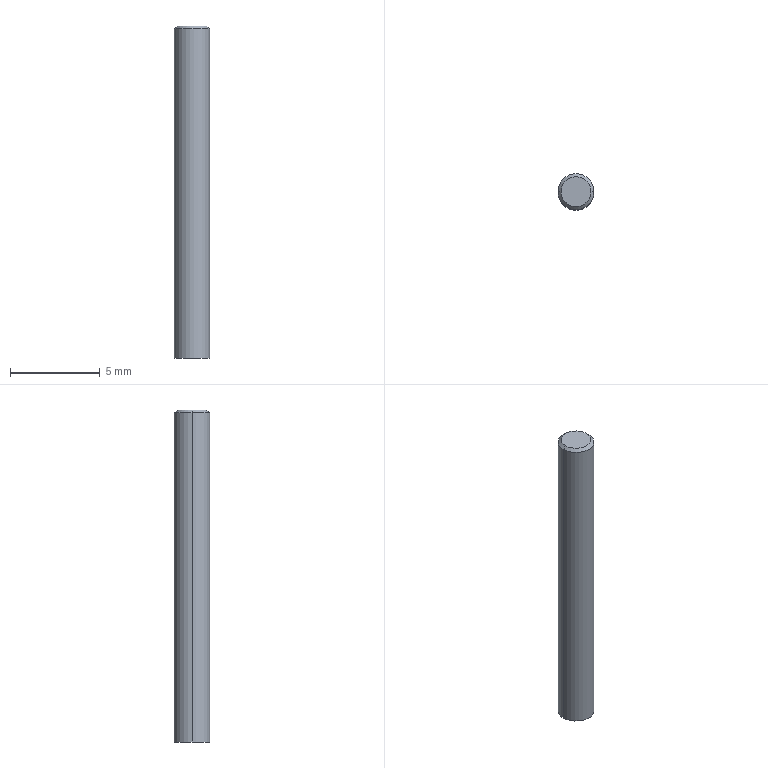Part | STEP file | rod_A_CJPS4_10_B_0_ | 1 solid | 6 faces | box 2 x 2 x 18.5 mm | volume 58.039 mm3 | cylinder 2 | cone 2 | plane 2 | commonest cylinder face diameters 2 x2
STEP:
#1=CARTESIAN_POINT('',(1.,0.,-11.));
#2=VERTEX_POINT('',#1);
#3=CARTESIAN_POINT('',(-1.,0.,-11.));
#4=VERTEX_POINT('',#3);
#5=CARTESIAN_POINT('',(0.,0.,-11.));
#6=DIRECTION('',(0.,0.,1.));
#7=DIRECTION('',(1.,0.,0.));
#8=AXIS2_PLACEMENT_3D('',#5,#6,#7);
#9=CIRCLE('',#8,1.);
#10=EDGE_CURVE('',#2,#4,#9,.T.);
#11=ORIENTED_EDGE('',*,*,#10,.T.);
#12=CARTESIAN_POINT('',(-1.,0.,7.335));
#13=VERTEX_POINT('',#12);
#14=CARTESIAN_POINT('',(-1.,0.,-11.));
#15=DIRECTION('',(0.,0.,1.));
#16=VECTOR('',#15,1000.);
#17=LINE('',#14,#16);
#18=EDGE_CURVE('',#4,#13,#17,.T.);
#19=ORIENTED_EDGE('',*,*,#18,.T.);
#20=CARTESIAN_POINT('',(1.,0.,7.335));
#21=VERTEX_POINT('',#20);
#22=CARTESIAN_POINT('',(0.,0.,7.335));
#23=DIRECTION('',(0.,0.,1.));
#24=DIRECTION('',(1.,0.,0.));
#25=AXIS2_PLACEMENT_3D('',#22,#23,#24);
#26=CIRCLE('',#25,1.);
#27=EDGE_CURVE('',#21,#13,#26,.T.);
#28=ORIENTED_EDGE('',*,*,#27,.F.);
#29=CARTESIAN_POINT('',(1.,0.,-11.));
#30=DIRECTION('',(0.,0.,1.));
#31=VECTOR('',#30,1000.);
#32=LINE('',#29,#31);
#33=EDGE_CURVE('',#2,#21,#32,.T.);
#34=ORIENTED_EDGE('',*,*,#33,.F.);
#35=EDGE_LOOP('',(#11,#19,#28,#34));
#36=FACE_OUTER_BOUND('',#35,.T.);
#37=CARTESIAN_POINT('',(0.,0.,-11.));
#38=DIRECTION('',(0.,0.,1.));
#39=DIRECTION('',(1.,0.,0.));
#40=AXIS2_PLACEMENT_3D('',#37,#38,#39);
#41=CYLINDRICAL_SURFACE('',#40,1.);
#42=ADVANCED_FACE('',(#36),#41,.T.);
#43=CARTESIAN_POINT('',(0.835,0.,7.5));
#44=VERTEX_POINT('',#43);
#45=CARTESIAN_POINT('',(-0.835,0.,7.5));
#46=VERTEX_POINT('',#45);
#47=CARTESIAN_POINT('',(0.,0.,7.5));
#48=DIRECTION('',(0.,0.,1.));
#49=DIRECTION('',(1.,0.,0.));
#50=AXIS2_PLACEMENT_3D('',#47,#48,#49);
#51=CIRCLE('',#50,0.835);
#52=EDGE_CURVE('',#44,#46,#51,.T.);
#53=ORIENTED_EDGE('',*,*,#52,.F.);
#54=CARTESIAN_POINT('',(1.,0.,7.335));
#55=DIRECTION('',(0.7071,0.,-0.7071));
#56=VECTOR('',#55,1000.);
#57=LINE('',#54,#56);
#58=EDGE_CURVE('',#44,#21,#57,.T.);
#59=ORIENTED_EDGE('',*,*,#58,.T.);
#60=ORIENTED_EDGE('',*,*,#27,.T.);
#61=CARTESIAN_POINT('',(-1.,0.,7.335));
#62=DIRECTION('',(-0.7071,0.,-0.7071));
#63=VECTOR('',#62,1000.);
#64=LINE('',#61,#63);
#65=EDGE_CURVE('',#46,#13,#64,.T.);
#66=ORIENTED_EDGE('',*,*,#65,.F.);
#67=EDGE_LOOP('',(#53,#59,#60,#66));
#68=FACE_OUTER_BOUND('',#67,.T.);
#69=CARTESIAN_POINT('',(0.,0.,7.335));
#70=DIRECTION('',(0.,0.,-1.));
#71=DIRECTION('',(-1.,0.,0.));
#72=AXIS2_PLACEMENT_3D('',#69,#70,#71);
#73=CONICAL_SURFACE('',#72,1.,0.7854);
#74=ADVANCED_FACE('',(#68),#73,.T.);
#75=CARTESIAN_POINT('',(0.,0.,7.5));
#76=DIRECTION('',(0.,0.,1.));
#77=DIRECTION('',(1.,0.,0.));
#78=AXIS2_PLACEMENT_3D('',#75,#76,#77);
#79=CIRCLE('',#78,0.835);
#80=EDGE_CURVE('',#46,#44,#79,.T.);
#81=ORIENTED_EDGE('',*,*,#80,.T.);
#82=ORIENTED_EDGE('',*,*,#52,.T.);
#83=EDGE_LOOP('',(#81,#82));
#84=FACE_OUTER_BOUND('',#83,.T.);
#85=CARTESIAN_POINT('',(0.,0.,7.5));
#86=DIRECTION('',(0.,0.,-1.));
#87=DIRECTION('',(-1.,0.,0.));
#88=AXIS2_PLACEMENT_3D('',#85,#86,#87);
#89=PLANE('',#88);
#90=ADVANCED_FACE('',(#84),#89,.F.);
#91=ORIENTED_EDGE('',*,*,#58,.F.);
#92=ORIENTED_EDGE('',*,*,#80,.F.);
#93=ORIENTED_EDGE('',*,*,#65,.T.);
#94=CARTESIAN_POINT('',(0.,0.,7.335));
#95=DIRECTION('',(0.,0.,1.));
#96=DIRECTION('',(1.,0.,0.));
#97=AXIS2_PLACEMENT_3D('',#94,#95,#96);
#98=CIRCLE('',#97,1.);
#99=EDGE_CURVE('',#13,#21,#98,.T.);
#100=ORIENTED_EDGE('',*,*,#99,.T.);
#101=EDGE_LOOP('',(#91,#92,#93,#100));
#102=FACE_OUTER_BOUND('',#101,.T.);
#103=CARTESIAN_POINT('',(0.,0.,7.335));
#104=DIRECTION('',(0.,0.,-1.));
#105=DIRECTION('',(-1.,0.,0.));
#106=AXIS2_PLACEMENT_3D('',#103,#104,#105);
#107=CONICAL_SURFACE('',#106,1.,0.7854);
#108=ADVANCED_FACE('',(#102),#107,.T.);
#109=ORIENTED_EDGE('',*,*,#18,.F.);
#110=CARTESIAN_POINT('',(0.,0.,-11.));
#111=DIRECTION('',(0.,0.,1.));
#112=DIRECTION('',(1.,0.,0.));
#113=AXIS2_PLACEMENT_3D('',#110,#111,#112);
#114=CIRCLE('',#113,1.);
#115=EDGE_CURVE('',#4,#2,#114,.T.);
#116=ORIENTED_EDGE('',*,*,#115,.T.);
#117=ORIENTED_EDGE('',*,*,#33,.T.);
#118=ORIENTED_EDGE('',*,*,#99,.F.);
#119=EDGE_LOOP('',(#109,#116,#117,#118));
#120=FACE_OUTER_BOUND('',#119,.T.);
#121=CARTESIAN_POINT('',(0.,0.,-11.));
#122=DIRECTION('',(0.,0.,1.));
#123=DIRECTION('',(1.,0.,0.));
#124=AXIS2_PLACEMENT_3D('',#121,#122,#123);
#125=CYLINDRICAL_SURFACE('',#124,1.);
#126=ADVANCED_FACE('',(#120),#125,.T.);
#127=ORIENTED_EDGE('',*,*,#10,.F.);
#128=ORIENTED_EDGE('',*,*,#115,.F.);
#129=EDGE_LOOP('',(#127,#128));
#130=FACE_OUTER_BOUND('',#129,.T.);
#131=CARTESIAN_POINT('',(0.,1.,-11.));
#132=DIRECTION('',(0.,0.,1.));
#133=DIRECTION('',(1.,0.,0.));
#134=AXIS2_PLACEMENT_3D('',#131,#132,#133);
#135=PLANE('',#134);
#136=ADVANCED_FACE('',(#130),#135,.F.);
#137=CLOSED_SHELL('',(#42,#74,#90,#108,#126,#136));
#138=MANIFOLD_SOLID_BREP('',#137);
#139=CARTESIAN_POINT('',(0.,0.,0.));
#140=DIRECTION('',(0.,0.,1.));
#141=DIRECTION('',(1.,0.,0.));
#142=AXIS2_PLACEMENT_3D('',#139,#140,#141);
#143=(LENGTH_UNIT()NAMED_UNIT(*)SI_UNIT(.MILLI.,.METRE.));
#144=UNCERTAINTY_MEASURE_WITH_UNIT(LENGTH_MEASURE(0.00001),#143,'','');
#145=(NAMED_UNIT(*)PLANE_ANGLE_UNIT()SI_UNIT($,.RADIAN.));
#146=(NAMED_UNIT(*)SI_UNIT($,.STERADIAN.)SOLID_ANGLE_UNIT());
#147=(GEOMETRIC_REPRESENTATION_CONTEXT(3)GLOBAL_UNCERTAINTY_ASSIGNED_CONTEXT((#144))GLOBAL_UNIT_ASSIGNED_CONTEXT((#143,#145,#146))REPRESENTATION_CONTEXT('',''));
#148=ADVANCED_BREP_SHAPE_REPRESENTATION('',(#138,#142),#147);